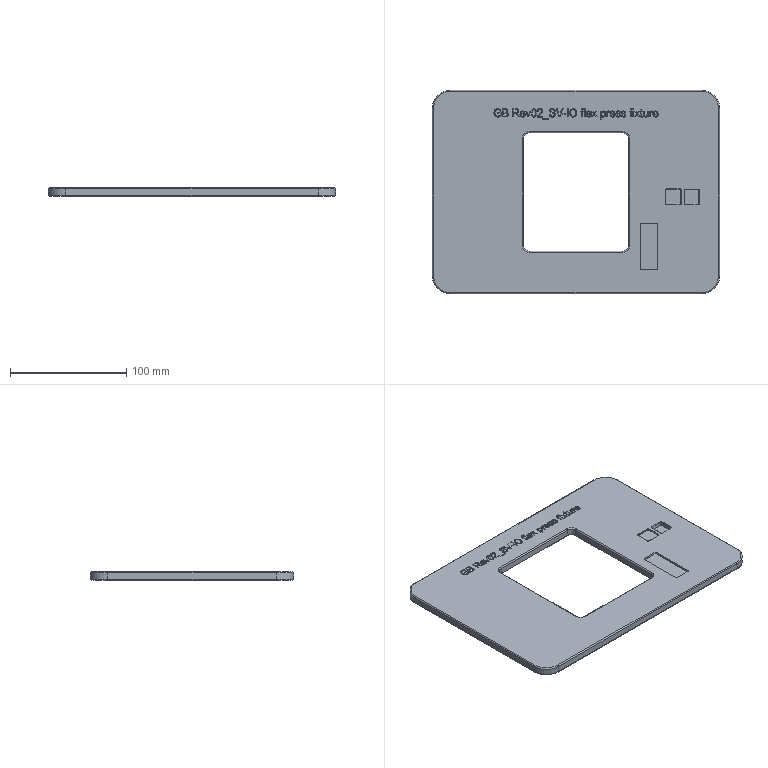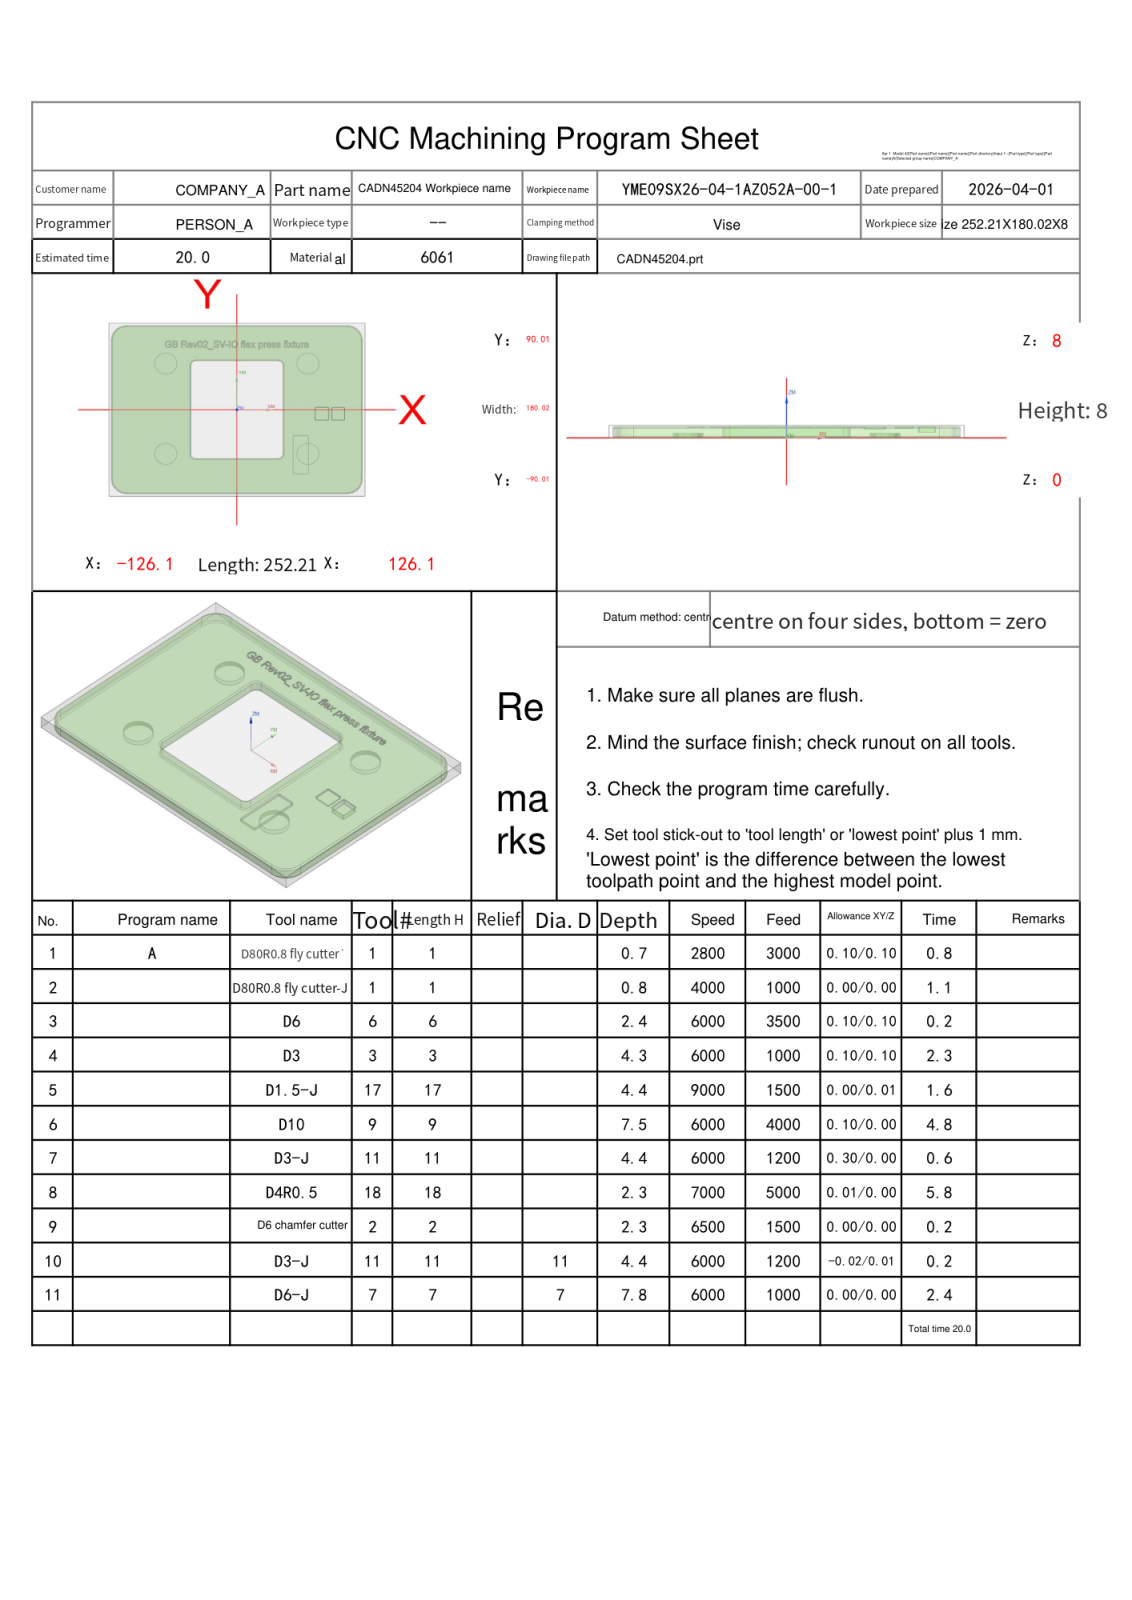NC program | NX | posted by the shop | part box 247.208 x 175.016 x 7.2 mm
Lines 1 to 874 of 29502:
%
O0001
(Machine time: 22.19 MIN)
(===Total Tool:9===)
(T1=D80R0.8 fly cutter D=80.  R=0.8  D-  H01 Z=7.2   )
(T6=D6      D=6.   R=0.   D-  H06 Z=5.6   )
(T3=D3      D=3.   R=0.   D-  H03 Z=3.66  )
(T17=D1.5-J D=1.5  R=0.   D-  H17 Z=3.56  )
(T9=D10     D=10.  R=0.   D-  H09 Z=0.5   )
(T11=D3-J   D=3.   R=0.   D-  H11 Z=3.56  )
(T18=D4R0.5 D=4.   R=0.5  D-  H18 Z=5.7   )
(T2=D6 chamfer cutter   D=6.   R=0.   D-  H02 Z=5.7   )
(T7=D6-J    D=6.   R=0.   D7  H07 Z=0.2   )
G80 G90 G17 G49 G40
G91 G28 Z0
M01
N1 T01 M06
(D80R0.8 fly cutter D=80. R=0.8 H=01 ce=0.10 di=0.10)
G00 G90 G54 X-175.701 Y63.603 M03 S2800
G43 H01 Z27.2
M08
Z9.75
G01 Z7.75 F3000.
X-163.701 Y63.604
X155.704 Y63.61
G02 X163.701 Y55.614 I-.003 J-8.
G01 Y11.679
G02 X155.705 Y3.683 I-8. J.004
G01 X-155.705 Y3.677
G03 X-163.701 Y-4.319 I.004 J-8.
G01 Y-48.253
G03 X-155.704 Y-56.25 I8. J.004
G01 X163.701 Y-56.244
X175.701 Y-56.243
Z9.75
G00 X-175.701 Y63.603
Z9.3
G01 Z7.3
X-163.701 Y63.604
X155.704 Y63.61
G02 X163.701 Y55.614 I-.003 J-8.
G01 Y11.679
G02 X155.705 Y3.683 I-8. J.004
G01 X-155.705 Y3.677
G03 X-163.701 Y-4.319 I.004 J-8.
G01 Y-48.253
G03 X-155.704 Y-56.25 I8. J.004
G01 X163.701 Y-56.244
X175.701 Y-56.243
Z9.3
G00 Z27.2
G91 G28 Z0.0
M05
M09
G91 G28 Z0.0
M01
N2 T01 M06
(D80R0.8 fly cutter-J D=80. R=0.8 H=01 ce=0.00 di=0.00)
G00 G90 G54 X-175.603 Y63.506 M03 S4000
G43 H01 Z27.2
M08
Z9.2
G01 Z7.2 F1000.
X-163.603
X155.607 Y63.512
G02 X163.603 Y55.515 I-.004 J-8.
G01 Y11.68
G02 X155.606 Y3.683 I-8. J.003
G01 X-155.607 Y3.677
G03 X-163.603 Y-4.319 I.004 J-8.
G01 Y-48.155
G03 X-155.607 Y-56.152 I8. J.004
G01 X163.603 Y-56.146
X175.603
Z9.2
G00 Z27.2
G91 G28 Z0.0
M05
M09
G91 G28 Z0.0
M01
N3 T06 M06
(D6  D=6. R=0. H=06 ce=0.10 di=0.10)
G00 G90 G54 X63.162 Y-55.388 M03 S6000
G43 H06 Z27.2
M08
Z7.7
G01 Y-34.119 Z7.143 F3500.
X62.762 Z7.133
Y-46.819 Z6.8
Y-59.519
X63.162
Y-34.119
X62.762
Y-46.819
X58.562
Y-63.719
X67.362
Y-29.919
X58.562
Y-46.819
Y-47.319
Z7.3
G00 Z7.7
X63.162 Y-55.388
Z7.3
G01 Y-34.119 Z6.743
X62.762 Z6.733
Y-46.819 Z6.4
Y-59.519
X63.162
Y-34.119
X62.762
Y-46.819
X58.562
Y-63.719
X67.362
Y-29.919
X58.562
Y-46.819
Y-47.319
Z6.9
G00 Z7.3
X63.162 Y-55.388
Z6.9
G01 Y-34.119 Z6.343
X62.762 Z6.333
Y-46.819 Z6.
Y-59.519
X63.162
Y-34.119
X62.762
Y-46.819
X58.562
Y-63.719
X67.362
Y-29.919
X58.562
Y-46.819
Y-47.319
Z6.5
G00 Z6.9
X63.162 Y-55.388
Z6.5
G01 Y-34.119 Z5.943
X62.762 Z5.933
Y-46.819 Z5.6
Y-59.519
X63.162
Y-34.119
X62.762
Y-46.819
X58.562
Y-63.719
X67.362
Y-29.919
X58.562
Y-46.819
Y-47.319
Z6.1
G00 Z27.2
G91 G28 Z0.0
M05
M09
G91 G28 Z0.0
M01
N4 T03 M06
(D3  D=3. R=0. H=03 ce=0.10 di=0.10)
G00 G90 G54 X86.326 Y-7.034 M03 S6000
G43 H03 Z27.2
M08
Z7.7
G01 X86.585 Z7.693 F1000.
Y-1.415 Z7.546
X80.944 Z7.398
Y-7.034 Z7.251
X86.585 Z7.104
Y-4.225 Z7.03
X84.485
Y-3.515
X83.044
Y-4.934
X84.485
Y-4.225
X86.585
Y-1.415
X80.944
Y-7.034
X86.585
Y-4.225
X88.685
Y.685
X78.844
Y-9.134
X88.685
Y-4.225
Y-3.725
Z7.53
G00 Z7.7
X86.326 Y-7.034
Z7.53
G01 X86.585 Z7.523
Y-1.415 Z7.376
X80.944 Z7.228
Y-7.034 Z7.081
X86.585 Z6.934
Y-4.225 Z6.86
X84.485
Y-3.515
X83.044
Y-4.934
X84.485
Y-4.225
X86.585
Y-1.415
X80.944
Y-7.034
X86.585
Y-4.225
X88.685
Y.685
X78.844
Y-9.134
X88.685
Y-4.225
Y-3.725
Z7.36
G00 Z7.53
X86.326 Y-7.034
Z7.36
G01 X86.585 Z7.353
Y-1.415 Z7.206
X80.944 Z7.058
Y-7.034 Z6.911
X86.585 Z6.764
Y-4.225 Z6.69
X84.485
Y-3.515
X83.044
Y-4.934
X84.485
Y-4.225
X86.585
Y-1.415
X80.944
Y-7.034
X86.585
Y-4.225
X88.685
Y.685
X78.844
Y-9.134
X88.685
Y-4.225
Y-3.725
Z7.19
G00 Z7.36
X86.326 Y-7.034
Z7.19
G01 X86.585 Z7.183
Y-1.415 Z7.036
X80.944 Z6.888
Y-7.034 Z6.741
X86.585 Z6.594
Y-4.225 Z6.52
X84.485
Y-3.515
X83.044
Y-4.934
X84.485
Y-4.225
X86.585
Y-1.415
X80.944
Y-7.034
X86.585
Y-4.225
X88.685
Y.685
X78.844
Y-9.134
X88.685
Y-4.225
Y-3.725
Z7.02
G00 Z7.19
X86.326 Y-7.034
Z7.02
G01 X86.585 Z7.013
Y-1.415 Z6.866
X80.944 Z6.718
Y-7.034 Z6.571
X86.585 Z6.424
Y-4.225 Z6.35
X84.485
Y-3.515
X83.044
Y-4.934
X84.485
Y-4.225
X86.585
Y-1.415
X80.944
Y-7.034
X86.585
Y-4.225
X88.685
Y.685
X78.844
Y-9.134
X88.685
Y-4.225
Y-3.725
Z6.85
G00 Z7.02
X86.326 Y-7.034
Z6.85
G01 X86.585 Z6.843
Y-1.415 Z6.696
X80.944 Z6.548
Y-7.034 Z6.401
X86.585 Z6.254
Y-4.225 Z6.18
X84.485
Y-3.515
X83.044
Y-4.934
X84.485
Y-4.225
X86.585
Y-1.415
X80.944
Y-7.034
X86.585
Y-4.225
X88.685
Y.685
X78.844
Y-9.134
X88.685
Y-4.225
Y-3.725
Z6.68
G00 Z27.2
G00 G90 X98.567 Y-7.034 M03 S6000
Z27.2
Z7.7
G01 X102.152 Z7.606 F1000.
Y-1.634 Z7.465
X97.39 Z7.34
Y-7.034 Z7.199
X102.152 Z7.074
Y-4.334 Z7.003
X100.052
Y-3.734
X99.49
Y-4.934
X100.052
Y-4.334
X102.152
Y-1.634
X97.39
Y-7.034
X102.152
Y-4.334
X104.252
Y.466
X95.29
Y-9.134
X104.252
Y-4.334
Y-3.834
Z7.503
G00 Z7.7
X98.567 Y-7.034
Z7.503
G01 X102.152 Z7.409
Y-1.634 Z7.268
X97.39 Z7.143
Y-7.034 Z7.002
X102.152 Z6.877
Y-4.334 Z6.806
X100.052
Y-3.734
X99.49
Y-4.934
X100.052
Y-4.334
X102.152
Y-1.634
X97.39
Y-7.034
X102.152
Y-4.334
X104.252
Y.466
X95.29
Y-9.134
X104.252
Y-4.334
Y-3.834
Z7.306
G00 Z7.503
X98.567 Y-7.034
Z7.306
G01 X102.152 Z7.213
Y-1.634 Z7.071
X97.39 Z6.947
Y-7.034 Z6.805
X102.152 Z6.68
Y-4.334 Z6.61
X100.052
Y-3.734
X99.49
Y-4.934
X100.052
Y-4.334
X102.152
Y-1.634
X97.39
Y-7.034
X102.152
Y-4.334
X104.252
Y.466
X95.29
Y-9.134
X104.252
Y-4.334
Y-3.834
Z7.11
G00 Z7.306
X98.567 Y-7.034
Z7.11
G01 X102.152 Z7.016
Y-1.634 Z6.874
X97.39 Z6.75
Y-7.034 Z6.608
X102.152 Z6.484
Y-4.334 Z6.413
X100.052
Y-3.734
X99.49
Y-4.934
X100.052
Y-4.334
X102.152
Y-1.634
X97.39
Y-7.034
X102.152
Y-4.334
X104.252
Y.466
X95.29
Y-9.134
X104.252
Y-4.334
Y-3.834
Z6.913
G00 Z7.11
X98.567 Y-7.034
Z6.913
G01 X102.152 Z6.819
Y-1.634 Z6.678
X97.39 Z6.553
Y-7.034 Z6.412
X102.152 Z6.287
Y-4.334 Z6.216
X100.052
Y-3.734
X99.49
Y-4.934
X100.052
Y-4.334
X102.152
Y-1.634
X97.39
Y-7.034
X102.152
Y-4.334
X104.252
Y.466
X95.29
Y-9.134
X104.252
Y-4.334
Y-3.834
Z6.716
G00 Z6.913
X98.567 Y-7.034
Z6.716
G01 X102.152 Z6.622
Y-1.634 Z6.481
X97.39 Z6.356
Y-7.034 Z6.215
X102.152 Z6.09
Y-4.334 Z6.019
X100.052
Y-3.734
X99.49
Y-4.934
X100.052
Y-4.334
X102.152
Y-1.634
X97.39
Y-7.034
X102.152
Y-4.334
X104.252
Y.466
X95.29
Y-9.134
X104.252
Y-4.334
Y-3.834
Z6.519
G00 Z6.716
X98.567 Y-7.034
Z6.519
G01 X102.152 Z6.426
Y-1.634 Z6.284
X97.39 Z6.159
Y-7.034 Z6.018
X102.152 Z5.893
Y-4.334 Z5.823
X100.052
Y-3.734
X99.49
Y-4.934
X100.052
Y-4.334
X102.152
Y-1.634
X97.39
Y-7.034
X102.152
Y-4.334
X104.252
Y.466
X95.29
Y-9.134
X104.252
Y-4.334
Y-3.834
Z6.323
G00 Z6.519
X98.567 Y-7.034
Z6.323
G01 X102.152 Z6.229
Y-1.634 Z6.087
X97.39 Z5.963
Y-7.034 Z5.821
X102.152 Z5.697
Y-4.334 Z5.626
X100.052
Y-3.734
X99.49
Y-4.934
X100.052
Y-4.334
X102.152
Y-1.634
X97.39
Y-7.034
X102.152
Y-4.334
X104.252
Y.466
X95.29
Y-9.134
X104.252
Y-4.334
Y-3.834
Z6.126
G00 Z6.323
X98.567 Y-7.034
Z6.126
G01 X102.152 Z6.032
Y-1.634 Z5.891
X97.39 Z5.766
Y-7.034 Z5.625
X102.152 Z5.5
Y-4.334 Z5.429
X100.052
Y-3.734
X99.49
Y-4.934
X100.052
Y-4.334
X102.152
Y-1.634
X97.39
Y-7.034
X102.152
Y-4.334
X104.252
Y.466
X95.29
Y-9.134
X104.252
Y-4.334
Y-3.834
Z5.929
G00 Z6.126
X98.567 Y-7.034
Z5.929
G01 X102.152 Z5.835
Y-1.634 Z5.694
X97.39 Z5.569
Y-7.034 Z5.428
X102.152 Z5.303
Y-4.334 Z5.232
X100.052
Y-3.734
X99.49
Y-4.934
X100.052
Y-4.334
X102.152
Y-1.634
X97.39
Y-7.034
X102.152
Y-4.334
X104.252
Y.466
X95.29
Y-9.134
X104.252
Y-4.334
Y-3.834
Z5.732
G00 Z5.929
X98.567 Y-7.034
Z5.732
G01 X102.152 Z5.639
Y-1.634 Z5.497
X97.39 Z5.372
Y-7.034 Z5.231
X102.152 Z5.106
Y-4.334 Z5.036
X100.052
Y-3.734
X99.49
Y-4.934
X100.052
Y-4.334
X102.152
Y-1.634
X97.39
Y-7.034
X102.152
Y-4.334
X104.252
Y.466
X95.29
Y-9.134
X104.252
Y-4.334
Y-3.834
Z5.536
G00 Z5.732
X98.567 Y-7.034
Z5.536
G01 X102.152 Z5.442
Y-1.634 Z5.3
X97.39 Z5.176
Y-7.034 Z5.034
X102.152 Z4.91
Y-4.334 Z4.839
X100.052
Y-3.734
X99.49
Y-4.934
X100.052
Y-4.334
X102.152
Y-1.634
X97.39
Y-7.034
X102.152
Y-4.334
X104.252
Y.466
X95.29
Y-9.134
X104.252
Y-4.334
Y-3.834
Z5.339
G00 Z5.536
X98.567 Y-7.034
Z5.339
G01 X102.152 Z5.245
Y-1.634 Z5.104
X97.39 Z4.979
Y-7.034 Z4.838
X102.152 Z4.713
Y-4.334 Z4.642
X100.052
Y-3.734
X99.49
Y-4.934
X100.052
Y-4.334
X102.152
Y-1.634
X97.39
Y-7.034
X102.152
Y-4.334
X104.252
Y.466
X95.29
Y-9.134
X104.252
Y-4.334
Y-3.834
Z5.142
G00 Z5.339
X98.567 Y-7.034
Z5.142
G01 X102.152 Z5.048
Y-1.634 Z4.907
X97.39 Z4.782
Y-7.034 Z4.641
X102.152 Z4.516
Y-4.334 Z4.445
X100.052
Y-3.734
X99.49
Y-4.934
X100.052
Y-4.334
X102.152
Y-1.634
X97.39
Y-7.034
X102.152
Y-4.334
X104.252
Y.466
X95.29
Y-9.134
X104.252
Y-4.334
Y-3.834
Z4.945
G00 Z5.142
X98.567 Y-7.034
Z4.945
G01 X102.152 Z4.852
Y-1.634 Z4.71
X97.39 Z4.585
Y-7.034 Z4.444
X102.152 Z4.319
Y-4.334 Z4.249
X100.052
Y-3.734
X99.49
Y-4.934
X100.052
Y-4.334
X102.152
Y-1.634
X97.39
Y-7.034
X102.152
Y-4.334
X104.252
Y.466
X95.29
Y-9.134
X104.252
Y-4.334
Y-3.834
Z4.749
G00 Z4.945
X98.567 Y-7.034
Z4.749
G01 X102.152 Z4.655
Y-1.634 Z4.513
X97.39 Z4.389
Y-7.034 Z4.247
X102.152 Z4.123
Y-4.334 Z4.052
X100.052
Y-3.734
X99.49
Y-4.934
X100.052
Y-4.334
X102.152
Y-1.634
X97.39
Y-7.034
X102.152
Y-4.334
X104.252
Y.466
X95.29
Y-9.134
X104.252
Y-4.334
Y-3.834
Z4.552
G00 Z4.749
X98.567 Y-7.034
Z4.552
G01 X102.152 Z4.458
Y-1.634 Z4.317
X97.39 Z4.192
Y-7.034 Z4.051
X102.152 Z3.926
Y-4.334 Z3.855
X100.052
Y-3.734
X99.49
Y-4.934
X100.052
Y-4.334
X102.152
Y-1.634
X97.39
Y-7.034
X102.152
Y-4.334
X104.252
Y.466
X95.29
Y-9.134
X104.252
Y-4.334
Y-3.834
Z4.355
G00 Z4.552
X98.567 Y-7.034
Z4.355
G01 X102.152 Z4.261
Y-1.634 Z4.12
X97.39 Z3.995
Y-7.034 Z3.854
X102.152 Z3.729
Y-4.334 Z3.658
X100.052
Y-3.734
X99.49
Y-4.934
X100.052
Y-4.334
X102.152
Y-1.634
X97.39
Y-7.034
X102.152
Y-4.334
X104.252
Y.466
X95.29
Y-9.134
X104.252
Y-4.334
Y-3.834
Z4.158
G00 Z27.2
G91 G28 Z0.0
M05
M09
G91 G28 Z0.0
M01